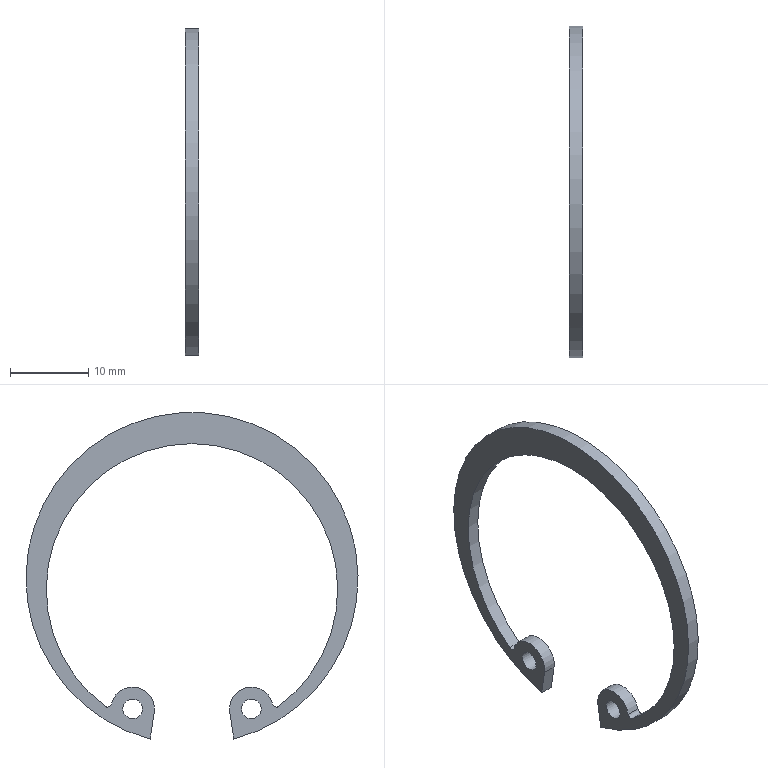Part | NX | features Retaining Ring C In-1_5003_010_BGBKB6203ZZ-40 2 | 1 solid | 12 faces | box 1.75 x 42.5 x 41.816 mm | volume 604.584 mm3 | cylinder 8 | plane 4 | commonest cylinder face diameters 1 x2 2.5 x2 5.594 x2 37.3 x1 42.5 x1
STEP:
#1=CARTESIAN_POINT('',(187.275,117.65,-163.699));
#2=VERTEX_POINT('',#1);
#3=CARTESIAN_POINT('',(187.275,116.4,-163.699));
#4=DIRECTION('',(1.,0.,0.));
#5=DIRECTION('',(0.,1.,0.));
#6=AXIS2_PLACEMENT_3D('',#3,#4,#5);
#7=CIRCLE('',#6,1.25);
#8=EDGE_CURVE('',#2,#2,#7,.T.);
#9=ORIENTED_EDGE('',*,*,#8,.F.);
#10=EDGE_LOOP('',(#9));
#11=FACE_BOUND('',#10,.T.);
#12=CARTESIAN_POINT('',(187.275,119.166,-164.112));
#13=VERTEX_POINT('',#12);
#14=CARTESIAN_POINT('',(187.275,113.671,-163.085));
#15=VERTEX_POINT('',#14);
#16=CARTESIAN_POINT('',(187.275,116.4,-163.699));
#17=DIRECTION('',(1.,0.,0.));
#18=DIRECTION('',(0.,1.,0.));
#19=AXIS2_PLACEMENT_3D('',#16,#17,#18);
#20=CIRCLE('',#19,2.797);
#21=EDGE_CURVE('',#13,#15,#20,.T.);
#22=ORIENTED_EDGE('',*,*,#21,.T.);
#23=CARTESIAN_POINT('',(187.275,112.886,-163.376));
#24=VERTEX_POINT('',#23);
#25=CARTESIAN_POINT('',(187.275,113.184,-162.975));
#26=DIRECTION('',(-1.,0.,0.));
#27=DIRECTION('',(0.,1.,0.));
#28=AXIS2_PLACEMENT_3D('',#25,#26,#27);
#29=CIRCLE('',#28,0.5);
#30=EDGE_CURVE('',#15,#24,#29,.T.);
#31=ORIENTED_EDGE('',*,*,#30,.T.);
#32=CARTESIAN_POINT('',(187.275,135.114,-163.376));
#33=VERTEX_POINT('',#32);
#34=CARTESIAN_POINT('',(187.275,124.,-148.4));
#35=DIRECTION('',(-1.,0.,0.));
#36=DIRECTION('',(0.,1.,0.));
#37=AXIS2_PLACEMENT_3D('',#34,#35,#36);
#38=CIRCLE('',#37,18.65);
#39=EDGE_CURVE('',#24,#33,#38,.T.);
#40=ORIENTED_EDGE('',*,*,#39,.T.);
#41=CARTESIAN_POINT('',(187.275,134.329,-163.085));
#42=VERTEX_POINT('',#41);
#43=CARTESIAN_POINT('',(187.275,134.816,-162.975));
#44=DIRECTION('',(-1.,0.,0.));
#45=DIRECTION('',(0.,-1.,0.));
#46=AXIS2_PLACEMENT_3D('',#43,#44,#45);
#47=CIRCLE('',#46,0.5);
#48=EDGE_CURVE('',#33,#42,#47,.T.);
#49=ORIENTED_EDGE('',*,*,#48,.T.);
#50=CARTESIAN_POINT('',(187.275,128.834,-164.112));
#51=VERTEX_POINT('',#50);
#52=CARTESIAN_POINT('',(187.275,131.6,-163.699));
#53=DIRECTION('',(1.,0.,0.));
#54=DIRECTION('',(0.,1.,0.));
#55=AXIS2_PLACEMENT_3D('',#52,#53,#54);
#56=CIRCLE('',#55,2.797);
#57=EDGE_CURVE('',#42,#51,#56,.T.);
#58=ORIENTED_EDGE('',*,*,#57,.T.);
#59=CARTESIAN_POINT('',(187.275,129.35,-167.566));
#60=VERTEX_POINT('',#59);
#61=CARTESIAN_POINT('',(187.275,128.834,-164.112));
#62=DIRECTION('',(0.,0.1478,-0.989));
#63=VECTOR('',#62,1000.);
#64=LINE('',#61,#63);
#65=EDGE_CURVE('',#51,#60,#64,.T.);
#66=ORIENTED_EDGE('',*,*,#65,.T.);
#67=CARTESIAN_POINT('',(187.275,118.65,-167.566));
#68=VERTEX_POINT('',#67);
#69=CARTESIAN_POINT('',(187.275,124.,-147.));
#70=DIRECTION('',(1.,0.,0.));
#71=DIRECTION('',(0.,1.,0.));
#72=AXIS2_PLACEMENT_3D('',#69,#70,#71);
#73=CIRCLE('',#72,21.25);
#74=EDGE_CURVE('',#60,#68,#73,.T.);
#75=ORIENTED_EDGE('',*,*,#74,.T.);
#76=CARTESIAN_POINT('',(187.275,119.166,-164.112));
#77=DIRECTION('',(0.,0.1478,0.989));
#78=VECTOR('',#77,1000.);
#79=LINE('',#76,#78);
#80=EDGE_CURVE('',#68,#13,#79,.T.);
#81=ORIENTED_EDGE('',*,*,#80,.T.);
#82=EDGE_LOOP('',(#22,#31,#40,#49,#58,#66,#75,#81));
#83=FACE_BOUND('',#82,.T.);
#84=CARTESIAN_POINT('',(187.275,132.85,-163.699));
#85=VERTEX_POINT('',#84);
#86=CARTESIAN_POINT('',(187.275,131.6,-163.699));
#87=DIRECTION('',(1.,0.,0.));
#88=DIRECTION('',(0.,1.,0.));
#89=AXIS2_PLACEMENT_3D('',#86,#87,#88);
#90=CIRCLE('',#89,1.25);
#91=EDGE_CURVE('',#85,#85,#90,.T.);
#92=ORIENTED_EDGE('',*,*,#91,.F.);
#93=EDGE_LOOP('',(#92));
#94=FACE_BOUND('',#93,.T.);
#95=CARTESIAN_POINT('',(187.275,116.4,-163.699));
#96=DIRECTION('',(1.,0.,0.));
#97=DIRECTION('',(0.,1.,0.));
#98=AXIS2_PLACEMENT_3D('',#95,#96,#97);
#99=PLANE('',#98);
#100=ADVANCED_FACE('',(#11,#83,#94),#99,.T.);
#101=CARTESIAN_POINT('',(185.525,119.166,-164.112));
#102=VERTEX_POINT('',#101);
#103=CARTESIAN_POINT('',(185.525,113.671,-163.085));
#104=VERTEX_POINT('',#103);
#105=CARTESIAN_POINT('',(185.525,116.4,-163.699));
#106=DIRECTION('',(1.,0.,0.));
#107=DIRECTION('',(0.,1.,0.));
#108=AXIS2_PLACEMENT_3D('',#105,#106,#107);
#109=CIRCLE('',#108,2.797);
#110=EDGE_CURVE('',#102,#104,#109,.T.);
#111=ORIENTED_EDGE('',*,*,#110,.F.);
#112=CARTESIAN_POINT('',(185.525,118.65,-167.566));
#113=VERTEX_POINT('',#112);
#114=CARTESIAN_POINT('',(185.525,119.166,-164.112));
#115=DIRECTION('',(0.,0.1478,0.989));
#116=VECTOR('',#115,1000.);
#117=LINE('',#114,#116);
#118=EDGE_CURVE('',#113,#102,#117,.T.);
#119=ORIENTED_EDGE('',*,*,#118,.F.);
#120=CARTESIAN_POINT('',(185.525,129.35,-167.566));
#121=VERTEX_POINT('',#120);
#122=CARTESIAN_POINT('',(185.525,124.,-147.));
#123=DIRECTION('',(1.,0.,0.));
#124=DIRECTION('',(0.,1.,0.));
#125=AXIS2_PLACEMENT_3D('',#122,#123,#124);
#126=CIRCLE('',#125,21.25);
#127=EDGE_CURVE('',#121,#113,#126,.T.);
#128=ORIENTED_EDGE('',*,*,#127,.F.);
#129=CARTESIAN_POINT('',(185.525,128.834,-164.112));
#130=VERTEX_POINT('',#129);
#131=CARTESIAN_POINT('',(185.525,128.834,-164.112));
#132=DIRECTION('',(0.,0.1478,-0.989));
#133=VECTOR('',#132,1000.);
#134=LINE('',#131,#133);
#135=EDGE_CURVE('',#130,#121,#134,.T.);
#136=ORIENTED_EDGE('',*,*,#135,.F.);
#137=CARTESIAN_POINT('',(185.525,134.329,-163.085));
#138=VERTEX_POINT('',#137);
#139=CARTESIAN_POINT('',(185.525,131.6,-163.699));
#140=DIRECTION('',(1.,0.,0.));
#141=DIRECTION('',(0.,1.,0.));
#142=AXIS2_PLACEMENT_3D('',#139,#140,#141);
#143=CIRCLE('',#142,2.797);
#144=EDGE_CURVE('',#138,#130,#143,.T.);
#145=ORIENTED_EDGE('',*,*,#144,.F.);
#146=CARTESIAN_POINT('',(185.525,135.114,-163.376));
#147=VERTEX_POINT('',#146);
#148=CARTESIAN_POINT('',(185.525,134.816,-162.975));
#149=DIRECTION('',(-1.,0.,0.));
#150=DIRECTION('',(0.,-1.,0.));
#151=AXIS2_PLACEMENT_3D('',#148,#149,#150);
#152=CIRCLE('',#151,0.5);
#153=EDGE_CURVE('',#147,#138,#152,.T.);
#154=ORIENTED_EDGE('',*,*,#153,.F.);
#155=CARTESIAN_POINT('',(185.525,112.886,-163.376));
#156=VERTEX_POINT('',#155);
#157=CARTESIAN_POINT('',(185.525,124.,-148.4));
#158=DIRECTION('',(-1.,0.,0.));
#159=DIRECTION('',(0.,1.,0.));
#160=AXIS2_PLACEMENT_3D('',#157,#158,#159);
#161=CIRCLE('',#160,18.65);
#162=EDGE_CURVE('',#156,#147,#161,.T.);
#163=ORIENTED_EDGE('',*,*,#162,.F.);
#164=CARTESIAN_POINT('',(185.525,113.184,-162.975));
#165=DIRECTION('',(-1.,0.,0.));
#166=DIRECTION('',(0.,1.,0.));
#167=AXIS2_PLACEMENT_3D('',#164,#165,#166);
#168=CIRCLE('',#167,0.5);
#169=EDGE_CURVE('',#104,#156,#168,.T.);
#170=ORIENTED_EDGE('',*,*,#169,.F.);
#171=EDGE_LOOP('',(#111,#119,#128,#136,#145,#154,#163,#170));
#172=FACE_BOUND('',#171,.T.);
#173=CARTESIAN_POINT('',(185.525,117.65,-163.699));
#174=VERTEX_POINT('',#173);
#175=CARTESIAN_POINT('',(185.525,116.4,-163.699));
#176=DIRECTION('',(1.,0.,0.));
#177=DIRECTION('',(0.,1.,0.));
#178=AXIS2_PLACEMENT_3D('',#175,#176,#177);
#179=CIRCLE('',#178,1.25);
#180=EDGE_CURVE('',#174,#174,#179,.T.);
#181=ORIENTED_EDGE('',*,*,#180,.T.);
#182=EDGE_LOOP('',(#181));
#183=FACE_BOUND('',#182,.T.);
#184=CARTESIAN_POINT('',(185.525,132.85,-163.699));
#185=VERTEX_POINT('',#184);
#186=CARTESIAN_POINT('',(185.525,131.6,-163.699));
#187=DIRECTION('',(1.,0.,0.));
#188=DIRECTION('',(0.,1.,0.));
#189=AXIS2_PLACEMENT_3D('',#186,#187,#188);
#190=CIRCLE('',#189,1.25);
#191=EDGE_CURVE('',#185,#185,#190,.T.);
#192=ORIENTED_EDGE('',*,*,#191,.T.);
#193=EDGE_LOOP('',(#192));
#194=FACE_BOUND('',#193,.T.);
#195=CARTESIAN_POINT('',(185.525,116.4,-163.699));
#196=DIRECTION('',(1.,0.,0.));
#197=DIRECTION('',(0.,1.,0.));
#198=AXIS2_PLACEMENT_3D('',#195,#196,#197);
#199=PLANE('',#198);
#200=ADVANCED_FACE('',(#172,#183,#194),#199,.F.);
#201=ORIENTED_EDGE('',*,*,#110,.T.);
#202=CARTESIAN_POINT('',(187.275,113.671,-163.085));
#203=DIRECTION('',(-1.,0.,0.));
#204=VECTOR('',#203,1000.);
#205=LINE('',#202,#204);
#206=EDGE_CURVE('',#15,#104,#205,.T.);
#207=ORIENTED_EDGE('',*,*,#206,.F.);
#208=ORIENTED_EDGE('',*,*,#21,.F.);
#209=CARTESIAN_POINT('',(187.275,119.166,-164.112));
#210=DIRECTION('',(-1.,0.,0.));
#211=VECTOR('',#210,1000.);
#212=LINE('',#209,#211);
#213=EDGE_CURVE('',#13,#102,#212,.T.);
#214=ORIENTED_EDGE('',*,*,#213,.T.);
#215=EDGE_LOOP('',(#201,#207,#208,#214));
#216=FACE_BOUND('',#215,.T.);
#217=CARTESIAN_POINT('',(187.275,116.4,-163.699));
#218=DIRECTION('',(-1.,0.,0.));
#219=DIRECTION('',(0.,-1.,0.));
#220=AXIS2_PLACEMENT_3D('',#217,#218,#219);
#221=CYLINDRICAL_SURFACE('',#220,2.797);
#222=ADVANCED_FACE('',(#216),#221,.T.);
#223=ORIENTED_EDGE('',*,*,#169,.T.);
#224=CARTESIAN_POINT('',(187.275,112.886,-163.376));
#225=DIRECTION('',(-1.,0.,0.));
#226=VECTOR('',#225,1000.);
#227=LINE('',#224,#226);
#228=EDGE_CURVE('',#24,#156,#227,.T.);
#229=ORIENTED_EDGE('',*,*,#228,.F.);
#230=ORIENTED_EDGE('',*,*,#30,.F.);
#231=ORIENTED_EDGE('',*,*,#206,.T.);
#232=EDGE_LOOP('',(#223,#229,#230,#231));
#233=FACE_BOUND('',#232,.T.);
#234=CARTESIAN_POINT('',(187.275,113.184,-162.975));
#235=DIRECTION('',(-1.,0.,0.));
#236=DIRECTION('',(0.,-1.,0.));
#237=AXIS2_PLACEMENT_3D('',#234,#235,#236);
#238=CYLINDRICAL_SURFACE('',#237,0.5);
#239=ADVANCED_FACE('',(#233),#238,.F.);
#240=ORIENTED_EDGE('',*,*,#162,.T.);
#241=CARTESIAN_POINT('',(187.275,135.114,-163.376));
#242=DIRECTION('',(-1.,0.,0.));
#243=VECTOR('',#242,1000.);
#244=LINE('',#241,#243);
#245=EDGE_CURVE('',#33,#147,#244,.T.);
#246=ORIENTED_EDGE('',*,*,#245,.F.);
#247=ORIENTED_EDGE('',*,*,#39,.F.);
#248=ORIENTED_EDGE('',*,*,#228,.T.);
#249=EDGE_LOOP('',(#240,#246,#247,#248));
#250=FACE_BOUND('',#249,.T.);
#251=CARTESIAN_POINT('',(187.275,124.,-148.4));
#252=DIRECTION('',(-1.,0.,0.));
#253=DIRECTION('',(0.,-1.,0.));
#254=AXIS2_PLACEMENT_3D('',#251,#252,#253);
#255=CYLINDRICAL_SURFACE('',#254,18.65);
#256=ADVANCED_FACE('',(#250),#255,.F.);
#257=ORIENTED_EDGE('',*,*,#153,.T.);
#258=CARTESIAN_POINT('',(187.275,134.329,-163.085));
#259=DIRECTION('',(-1.,0.,0.));
#260=VECTOR('',#259,1000.);
#261=LINE('',#258,#260);
#262=EDGE_CURVE('',#42,#138,#261,.T.);
#263=ORIENTED_EDGE('',*,*,#262,.F.);
#264=ORIENTED_EDGE('',*,*,#48,.F.);
#265=ORIENTED_EDGE('',*,*,#245,.T.);
#266=EDGE_LOOP('',(#257,#263,#264,#265));
#267=FACE_BOUND('',#266,.T.);
#268=CARTESIAN_POINT('',(187.275,134.816,-162.975));
#269=DIRECTION('',(-1.,0.,0.));
#270=DIRECTION('',(0.,-1.,0.));
#271=AXIS2_PLACEMENT_3D('',#268,#269,#270);
#272=CYLINDRICAL_SURFACE('',#271,0.5);
#273=ADVANCED_FACE('',(#267),#272,.F.);
#274=ORIENTED_EDGE('',*,*,#144,.T.);
#275=CARTESIAN_POINT('',(187.275,128.834,-164.112));
#276=DIRECTION('',(-1.,0.,0.));
#277=VECTOR('',#276,1000.);
#278=LINE('',#275,#277);
#279=EDGE_CURVE('',#51,#130,#278,.T.);
#280=ORIENTED_EDGE('',*,*,#279,.F.);
#281=ORIENTED_EDGE('',*,*,#57,.F.);
#282=ORIENTED_EDGE('',*,*,#262,.T.);
#283=EDGE_LOOP('',(#274,#280,#281,#282));
#284=FACE_BOUND('',#283,.T.);
#285=CARTESIAN_POINT('',(187.275,131.6,-163.699));
#286=DIRECTION('',(-1.,0.,0.));
#287=DIRECTION('',(0.,-1.,0.));
#288=AXIS2_PLACEMENT_3D('',#285,#286,#287);
#289=CYLINDRICAL_SURFACE('',#288,2.797);
#290=ADVANCED_FACE('',(#284),#289,.T.);
#291=ORIENTED_EDGE('',*,*,#135,.T.);
#292=CARTESIAN_POINT('',(187.275,129.35,-167.566));
#293=DIRECTION('',(-1.,0.,0.));
#294=VECTOR('',#293,1000.);
#295=LINE('',#292,#294);
#296=EDGE_CURVE('',#60,#121,#295,.T.);
#297=ORIENTED_EDGE('',*,*,#296,.F.);
#298=ORIENTED_EDGE('',*,*,#65,.F.);
#299=ORIENTED_EDGE('',*,*,#279,.T.);
#300=EDGE_LOOP('',(#291,#297,#298,#299));
#301=FACE_BOUND('',#300,.T.);
#302=CARTESIAN_POINT('',(187.275,128.834,-164.112));
#303=DIRECTION('',(0.,0.989,0.1478));
#304=DIRECTION('',(0.,-0.1478,0.989));
#305=AXIS2_PLACEMENT_3D('',#302,#303,#304);
#306=PLANE('',#305);
#307=ADVANCED_FACE('',(#301),#306,.F.);
#308=ORIENTED_EDGE('',*,*,#127,.T.);
#309=CARTESIAN_POINT('',(187.275,118.65,-167.566));
#310=DIRECTION('',(-1.,0.,0.));
#311=VECTOR('',#310,1000.);
#312=LINE('',#309,#311);
#313=EDGE_CURVE('',#68,#113,#312,.T.);
#314=ORIENTED_EDGE('',*,*,#313,.F.);
#315=ORIENTED_EDGE('',*,*,#74,.F.);
#316=ORIENTED_EDGE('',*,*,#296,.T.);
#317=EDGE_LOOP('',(#308,#314,#315,#316));
#318=FACE_BOUND('',#317,.T.);
#319=CARTESIAN_POINT('',(187.275,124.,-147.));
#320=DIRECTION('',(-1.,0.,0.));
#321=DIRECTION('',(0.,-1.,0.));
#322=AXIS2_PLACEMENT_3D('',#319,#320,#321);
#323=CYLINDRICAL_SURFACE('',#322,21.25);
#324=ADVANCED_FACE('',(#318),#323,.T.);
#325=ORIENTED_EDGE('',*,*,#118,.T.);
#326=ORIENTED_EDGE('',*,*,#213,.F.);
#327=ORIENTED_EDGE('',*,*,#80,.F.);
#328=ORIENTED_EDGE('',*,*,#313,.T.);
#329=EDGE_LOOP('',(#325,#326,#327,#328));
#330=FACE_BOUND('',#329,.T.);
#331=CARTESIAN_POINT('',(187.275,119.166,-164.112));
#332=DIRECTION('',(0.,-0.989,0.1478));
#333=DIRECTION('',(0.,-0.1478,-0.989));
#334=AXIS2_PLACEMENT_3D('',#331,#332,#333);
#335=PLANE('',#334);
#336=ADVANCED_FACE('',(#330),#335,.F.);
#337=ORIENTED_EDGE('',*,*,#8,.T.);
#338=EDGE_LOOP('',(#337));
#339=FACE_BOUND('',#338,.T.);
#340=ORIENTED_EDGE('',*,*,#180,.F.);
#341=EDGE_LOOP('',(#340));
#342=FACE_BOUND('',#341,.T.);
#343=CARTESIAN_POINT('',(187.275,116.4,-163.699));
#344=DIRECTION('',(-1.,0.,0.));
#345=DIRECTION('',(0.,-1.,0.));
#346=AXIS2_PLACEMENT_3D('',#343,#344,#345);
#347=CYLINDRICAL_SURFACE('',#346,1.25);
#348=ADVANCED_FACE('',(#339,#342),#347,.F.);
#349=ORIENTED_EDGE('',*,*,#91,.T.);
#350=EDGE_LOOP('',(#349));
#351=FACE_BOUND('',#350,.T.);
#352=ORIENTED_EDGE('',*,*,#191,.F.);
#353=EDGE_LOOP('',(#352));
#354=FACE_BOUND('',#353,.T.);
#355=CARTESIAN_POINT('',(187.275,131.6,-163.699));
#356=DIRECTION('',(-1.,0.,0.));
#357=DIRECTION('',(0.,-1.,0.));
#358=AXIS2_PLACEMENT_3D('',#355,#356,#357);
#359=CYLINDRICAL_SURFACE('',#358,1.25);
#360=ADVANCED_FACE('',(#351,#354),#359,.F.);
#361=CLOSED_SHELL('',(#100,#200,#222,#239,#256,#273,#290,#307,#324,#336,#348,#360));
#362=MANIFOLD_SOLID_BREP('',#361);
#363=(LENGTH_UNIT()NAMED_UNIT(*)SI_UNIT(.MILLI.,.METRE.));
#364=UNCERTAINTY_MEASURE_WITH_UNIT(LENGTH_MEASURE(0.00001),#363,'','');
#365=(NAMED_UNIT(*)PLANE_ANGLE_UNIT()SI_UNIT($,.RADIAN.));
#366=(NAMED_UNIT(*)SI_UNIT($,.STERADIAN.)SOLID_ANGLE_UNIT());
#367=(GEOMETRIC_REPRESENTATION_CONTEXT(3)GLOBAL_UNCERTAINTY_ASSIGNED_CONTEXT((#364))GLOBAL_UNIT_ASSIGNED_CONTEXT((#363,#365,#366))REPRESENTATION_CONTEXT('',''));
#368=ADVANCED_BREP_SHAPE_REPRESENTATION('',(#362),#367);